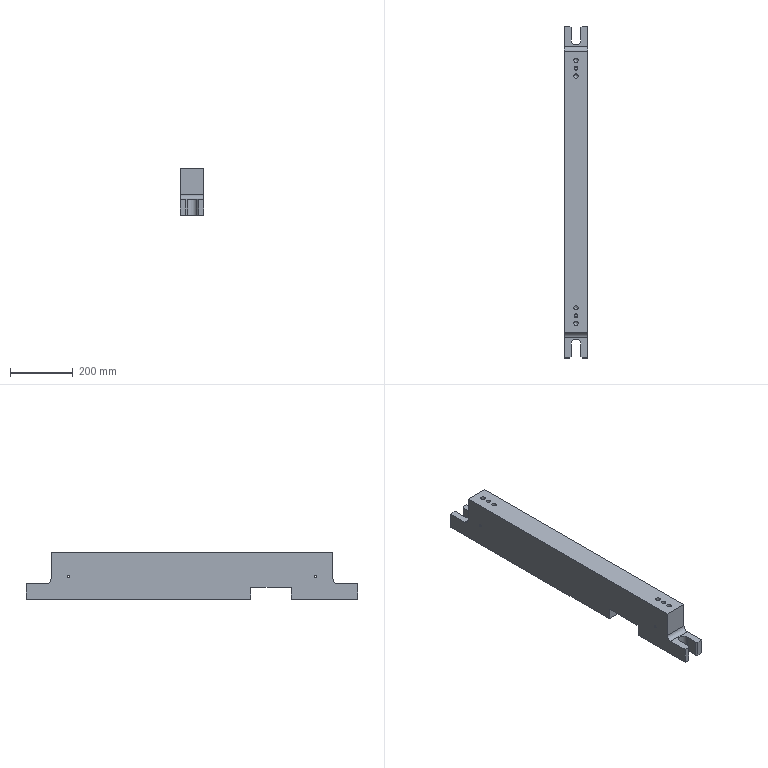Part | STEP file | 1_id1218_x_t | 1 solid | 52 faces | box 75 x 1060 x 149.325 mm | volume 10050016 mm3 | plane 26 | cylinder 16 | cone 10 | commonest cylinder face diameters 12.7 x4 14 x4 8 x2 10.716 x2 30 x2 31.75 x2